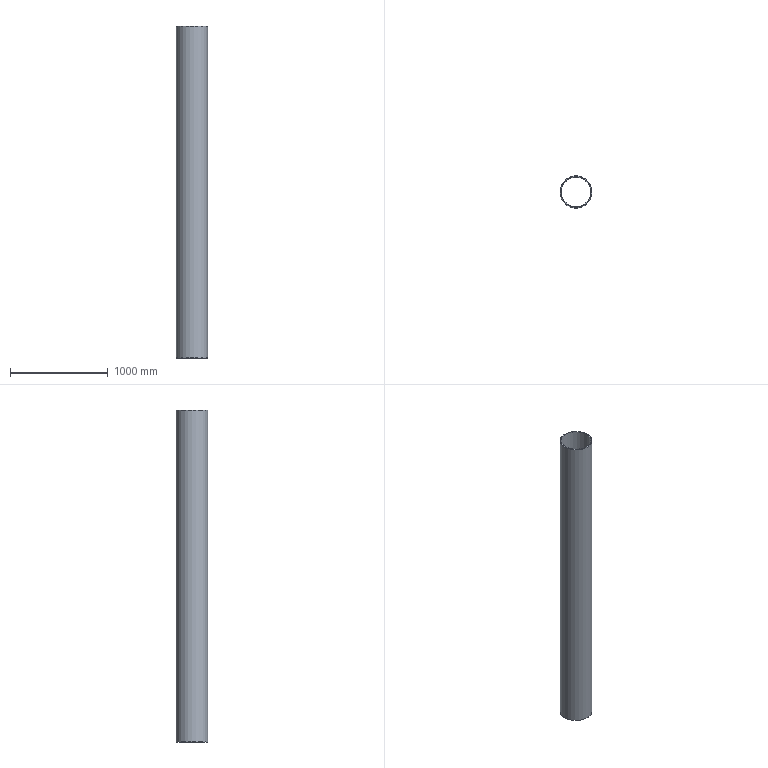Part | NX | features CHAMFER 1, CYLINDER 1, DATUM_CSYS 1, SHELL 1 | 1 solid | 6 faces | box 325 x 325 x 3398 mm | volume 27057214 mm3 | plane 2 | cylinder 2 | cone 2 | commonest cylinder face diameters 309 x1 325 x1
STEP:
#1=CARTESIAN_POINT('',(158.17,0.,3397.502));
#2=VERTEX_POINT('',#1);
#3=CARTESIAN_POINT('',(0.,0.,3397.502));
#4=DIRECTION('',(0.,0.,1.));
#5=DIRECTION('',(1.,0.,0.));
#6=AXIS2_PLACEMENT_3D('',#3,#4,#5);
#7=CIRCLE('',#6,158.17);
#8=EDGE_CURVE('',#2,#2,#7,.T.);
#9=ORIENTED_EDGE('',*,*,#8,.T.);
#10=EDGE_LOOP('',(#9));
#11=FACE_BOUND('',#10,.T.);
#12=CARTESIAN_POINT('',(154.5,0.,3397.502));
#13=VERTEX_POINT('',#12);
#14=CARTESIAN_POINT('',(0.,0.,3397.502));
#15=DIRECTION('',(0.,0.,1.));
#16=DIRECTION('',(1.,0.,0.));
#17=AXIS2_PLACEMENT_3D('',#14,#15,#16);
#18=CIRCLE('',#17,154.5);
#19=EDGE_CURVE('',#13,#13,#18,.F.);
#20=ORIENTED_EDGE('',*,*,#19,.T.);
#21=EDGE_LOOP('',(#20));
#22=FACE_BOUND('',#21,.T.);
#23=CARTESIAN_POINT('',(0.,0.,3397.502));
#24=DIRECTION('',(0.,0.,1.));
#25=DIRECTION('',(1.,0.,0.));
#26=AXIS2_PLACEMENT_3D('',#23,#24,#25);
#27=PLANE('',#26);
#28=ADVANCED_FACE('',(#11,#22),#27,.T.);
#29=CARTESIAN_POINT('',(-158.17,0.,0.));
#30=VERTEX_POINT('',#29);
#31=CARTESIAN_POINT('',(0.,0.,0.));
#32=DIRECTION('',(0.,0.,-1.));
#33=DIRECTION('',(-1.,0.,0.));
#34=AXIS2_PLACEMENT_3D('',#31,#32,#33);
#35=CIRCLE('',#34,158.17);
#36=EDGE_CURVE('',#30,#30,#35,.T.);
#37=ORIENTED_EDGE('',*,*,#36,.T.);
#38=EDGE_LOOP('',(#37));
#39=FACE_BOUND('',#38,.T.);
#40=CARTESIAN_POINT('',(-154.5,0.,0.));
#41=VERTEX_POINT('',#40);
#42=CARTESIAN_POINT('',(0.,0.,0.));
#43=DIRECTION('',(0.,0.,-1.));
#44=DIRECTION('',(-1.,0.,0.));
#45=AXIS2_PLACEMENT_3D('',#42,#43,#44);
#46=CIRCLE('',#45,154.5);
#47=EDGE_CURVE('',#41,#41,#46,.F.);
#48=ORIENTED_EDGE('',*,*,#47,.T.);
#49=EDGE_LOOP('',(#48));
#50=FACE_BOUND('',#49,.T.);
#51=CARTESIAN_POINT('',(0.,0.,0.));
#52=DIRECTION('',(0.,0.,-1.));
#53=DIRECTION('',(-1.,0.,0.));
#54=AXIS2_PLACEMENT_3D('',#51,#52,#53);
#55=PLANE('',#54);
#56=ADVANCED_FACE('',(#39,#50),#55,.T.);
#57=CARTESIAN_POINT('',(-162.5,0.,2.5));
#58=VERTEX_POINT('',#57);
#59=CARTESIAN_POINT('',(0.,0.,2.5));
#60=DIRECTION('',(0.,0.,-1.));
#61=DIRECTION('',(-1.,0.,0.));
#62=AXIS2_PLACEMENT_3D('',#59,#60,#61);
#63=CIRCLE('',#62,162.5);
#64=EDGE_CURVE('',#58,#58,#63,.F.);
#65=ORIENTED_EDGE('',*,*,#64,.T.);
#66=EDGE_LOOP('',(#65));
#67=FACE_BOUND('',#66,.T.);
#68=CARTESIAN_POINT('',(162.5,0.,3395.002));
#69=VERTEX_POINT('',#68);
#70=CARTESIAN_POINT('',(0.,0.,3395.002));
#71=DIRECTION('',(0.,0.,1.));
#72=DIRECTION('',(1.,0.,0.));
#73=AXIS2_PLACEMENT_3D('',#70,#71,#72);
#74=CIRCLE('',#73,162.5);
#75=EDGE_CURVE('',#69,#69,#74,.F.);
#76=ORIENTED_EDGE('',*,*,#75,.T.);
#77=EDGE_LOOP('',(#76));
#78=FACE_BOUND('',#77,.T.);
#79=CARTESIAN_POINT('',(0.,0.,0.));
#80=DIRECTION('',(0.,0.,1.));
#81=DIRECTION('',(1.,0.,0.));
#82=AXIS2_PLACEMENT_3D('',#79,#80,#81);
#83=CYLINDRICAL_SURFACE('',#82,162.5);
#84=ADVANCED_FACE('',(#67,#78),#83,.T.);
#85=ORIENTED_EDGE('',*,*,#19,.F.);
#86=EDGE_LOOP('',(#85));
#87=FACE_BOUND('',#86,.T.);
#88=ORIENTED_EDGE('',*,*,#47,.F.);
#89=EDGE_LOOP('',(#88));
#90=FACE_BOUND('',#89,.T.);
#91=CARTESIAN_POINT('',(0.,0.,0.));
#92=DIRECTION('',(0.,0.,1.));
#93=DIRECTION('',(1.,0.,0.));
#94=AXIS2_PLACEMENT_3D('',#91,#92,#93);
#95=CYLINDRICAL_SURFACE('',#94,154.5);
#96=ADVANCED_FACE('',(#87,#90),#95,.F.);
#97=ORIENTED_EDGE('',*,*,#36,.F.);
#98=EDGE_LOOP('',(#97));
#99=FACE_BOUND('',#98,.T.);
#100=ORIENTED_EDGE('',*,*,#64,.F.);
#101=EDGE_LOOP('',(#100));
#102=FACE_BOUND('',#101,.T.);
#103=CARTESIAN_POINT('',(0.,0.,2.5));
#104=DIRECTION('',(0.,0.,1.));
#105=DIRECTION('',(1.,0.,0.));
#106=AXIS2_PLACEMENT_3D('',#103,#104,#105);
#107=CONICAL_SURFACE('',#106,162.5,1.047);
#108=ADVANCED_FACE('',(#99,#102),#107,.T.);
#109=ORIENTED_EDGE('',*,*,#8,.F.);
#110=EDGE_LOOP('',(#109));
#111=FACE_BOUND('',#110,.T.);
#112=ORIENTED_EDGE('',*,*,#75,.F.);
#113=EDGE_LOOP('',(#112));
#114=FACE_BOUND('',#113,.T.);
#115=CARTESIAN_POINT('',(0.,0.,3395.002));
#116=DIRECTION('',(0.,0.,-1.));
#117=DIRECTION('',(-1.,0.,0.));
#118=AXIS2_PLACEMENT_3D('',#115,#116,#117);
#119=CONICAL_SURFACE('',#118,162.5,1.047);
#120=ADVANCED_FACE('',(#111,#114),#119,.T.);
#121=CLOSED_SHELL('',(#28,#56,#84,#96,#108,#120));
#122=MANIFOLD_SOLID_BREP('',#121);
#123=(LENGTH_UNIT()NAMED_UNIT(*)SI_UNIT(.MILLI.,.METRE.));
#124=UNCERTAINTY_MEASURE_WITH_UNIT(LENGTH_MEASURE(0.00001),#123,'','');
#125=(NAMED_UNIT(*)PLANE_ANGLE_UNIT()SI_UNIT($,.RADIAN.));
#126=(NAMED_UNIT(*)SI_UNIT($,.STERADIAN.)SOLID_ANGLE_UNIT());
#127=(GEOMETRIC_REPRESENTATION_CONTEXT(3)GLOBAL_UNCERTAINTY_ASSIGNED_CONTEXT((#124))GLOBAL_UNIT_ASSIGNED_CONTEXT((#123,#125,#126))REPRESENTATION_CONTEXT('',''));
#128=ADVANCED_BREP_SHAPE_REPRESENTATION('',(#122),#127);